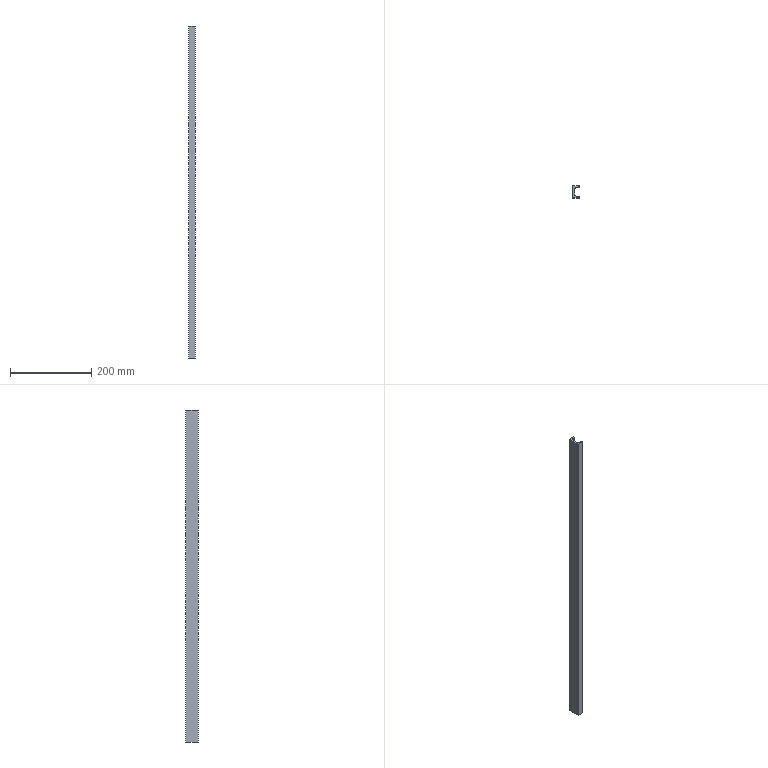Part | STEP file | DIN 1026-1 U 30x15 1785507254409 | 1 solid | 14 faces | box 15 x 30 x 815 mm | volume 180323 mm3 | plane 10 | cylinder 4 | commonest cylinder face diameters 4 x2 9 x2
STEP:
#1=CARTESIAN_POINT('',(4.,-6.066,815.));
#2=VERTEX_POINT('',#1);
#3=CARTESIAN_POINT('',(8.141,-10.551,815.));
#4=VERTEX_POINT('',#3);
#5=CARTESIAN_POINT('',(8.5,-6.066,815.));
#6=DIRECTION('',(0.,0.,1.));
#7=DIRECTION('',(-1.,0.,0.));
#8=AXIS2_PLACEMENT_3D('',#5,#6,#7);
#9=CIRCLE('',#8,4.5);
#10=EDGE_CURVE('',#2,#4,#9,.T.);
#11=ORIENTED_EDGE('',*,*,#10,.T.);
#12=CARTESIAN_POINT('',(8.141,-10.551,0.));
#13=VERTEX_POINT('',#12);
#14=CARTESIAN_POINT('',(8.141,-10.551,0.));
#15=DIRECTION('',(0.,0.,1.));
#16=VECTOR('',#15,10.);
#17=LINE('',#14,#16);
#18=EDGE_CURVE('',#13,#4,#17,.T.);
#19=ORIENTED_EDGE('',*,*,#18,.F.);
#20=CARTESIAN_POINT('',(4.,-6.066,0.));
#21=VERTEX_POINT('',#20);
#22=CARTESIAN_POINT('',(8.5,-6.066,0.));
#23=DIRECTION('',(0.,0.,1.));
#24=DIRECTION('',(-1.,0.,0.));
#25=AXIS2_PLACEMENT_3D('',#22,#23,#24);
#26=CIRCLE('',#25,4.5);
#27=EDGE_CURVE('',#21,#13,#26,.T.);
#28=ORIENTED_EDGE('',*,*,#27,.F.);
#29=CARTESIAN_POINT('',(4.,-6.066,0.));
#30=DIRECTION('',(0.,0.,1.));
#31=VECTOR('',#30,10.);
#32=LINE('',#29,#31);
#33=EDGE_CURVE('',#21,#2,#32,.T.);
#34=ORIENTED_EDGE('',*,*,#33,.T.);
#35=EDGE_LOOP('',(#11,#19,#28,#34));
#36=FACE_OUTER_BOUND('',#35,.T.);
#37=CARTESIAN_POINT('',(8.5,-6.066,0.));
#38=DIRECTION('',(0.,0.,1.));
#39=DIRECTION('',(-1.,0.,0.));
#40=AXIS2_PLACEMENT_3D('',#37,#38,#39);
#41=CYLINDRICAL_SURFACE('',#40,4.5);
#42=ADVANCED_FACE('',(#36),#41,.F.);
#43=CARTESIAN_POINT('',(13.159,-10.953,815.));
#44=VERTEX_POINT('',#43);
#45=CARTESIAN_POINT('',(7.403,-10.492,815.));
#46=DIRECTION('',(0.9968,-0.07975,0.));
#47=VECTOR('',#46,10.);
#48=LINE('',#45,#47);
#49=EDGE_CURVE('',#4,#44,#48,.T.);
#50=ORIENTED_EDGE('',*,*,#49,.T.);
#51=CARTESIAN_POINT('',(13.159,-10.953,0.));
#52=VERTEX_POINT('',#51);
#53=CARTESIAN_POINT('',(13.159,-10.953,0.));
#54=DIRECTION('',(0.,0.,1.));
#55=VECTOR('',#54,10.);
#56=LINE('',#53,#55);
#57=EDGE_CURVE('',#52,#44,#56,.T.);
#58=ORIENTED_EDGE('',*,*,#57,.F.);
#59=CARTESIAN_POINT('',(7.403,-10.492,0.));
#60=DIRECTION('',(0.9968,-0.07975,0.));
#61=VECTOR('',#60,10.);
#62=LINE('',#59,#61);
#63=EDGE_CURVE('',#13,#52,#62,.T.);
#64=ORIENTED_EDGE('',*,*,#63,.F.);
#65=ORIENTED_EDGE('',*,*,#18,.T.);
#66=EDGE_LOOP('',(#50,#58,#64,#65));
#67=FACE_OUTER_BOUND('',#66,.T.);
#68=CARTESIAN_POINT('',(8.141,-10.551,0.));
#69=DIRECTION('',(0.07975,0.9968,0.));
#70=DIRECTION('',(0.,0.,1.));
#71=AXIS2_PLACEMENT_3D('',#68,#69,#70);
#72=PLANE('',#71);
#73=ADVANCED_FACE('',(#67),#72,.T.);
#74=CARTESIAN_POINT('',(15.,-12.946,815.));
#75=VERTEX_POINT('',#74);
#76=CARTESIAN_POINT('',(13.,-12.946,815.));
#77=DIRECTION('',(0.,0.,-1.));
#78=DIRECTION('',(-1.,0.,0.));
#79=AXIS2_PLACEMENT_3D('',#76,#77,#78);
#80=CIRCLE('',#79,2.);
#81=EDGE_CURVE('',#44,#75,#80,.T.);
#82=ORIENTED_EDGE('',*,*,#81,.T.);
#83=CARTESIAN_POINT('',(15.,-12.946,0.));
#84=VERTEX_POINT('',#83);
#85=CARTESIAN_POINT('',(15.,-12.946,0.));
#86=DIRECTION('',(0.,0.,1.));
#87=VECTOR('',#86,10.);
#88=LINE('',#85,#87);
#89=EDGE_CURVE('',#84,#75,#88,.T.);
#90=ORIENTED_EDGE('',*,*,#89,.F.);
#91=CARTESIAN_POINT('',(13.,-12.946,0.));
#92=DIRECTION('',(0.,0.,-1.));
#93=DIRECTION('',(-1.,0.,0.));
#94=AXIS2_PLACEMENT_3D('',#91,#92,#93);
#95=CIRCLE('',#94,2.);
#96=EDGE_CURVE('',#52,#84,#95,.T.);
#97=ORIENTED_EDGE('',*,*,#96,.F.);
#98=ORIENTED_EDGE('',*,*,#57,.T.);
#99=EDGE_LOOP('',(#82,#90,#97,#98));
#100=FACE_OUTER_BOUND('',#99,.T.);
#101=CARTESIAN_POINT('',(13.,-12.946,0.));
#102=DIRECTION('',(0.,0.,1.));
#103=DIRECTION('',(-1.,0.,0.));
#104=AXIS2_PLACEMENT_3D('',#101,#102,#103);
#105=CYLINDRICAL_SURFACE('',#104,2.);
#106=ADVANCED_FACE('',(#100),#105,.T.);
#107=CARTESIAN_POINT('',(15.,-15.,815.));
#108=VERTEX_POINT('',#107);
#109=CARTESIAN_POINT('',(15.,-6.473,815.));
#110=DIRECTION('',(0.,-1.,0.));
#111=VECTOR('',#110,10.);
#112=LINE('',#109,#111);
#113=EDGE_CURVE('',#75,#108,#112,.T.);
#114=ORIENTED_EDGE('',*,*,#113,.T.);
#115=CARTESIAN_POINT('',(15.,-15.,0.));
#116=VERTEX_POINT('',#115);
#117=CARTESIAN_POINT('',(15.,-15.,0.));
#118=DIRECTION('',(0.,0.,1.));
#119=VECTOR('',#118,10.);
#120=LINE('',#117,#119);
#121=EDGE_CURVE('',#116,#108,#120,.T.);
#122=ORIENTED_EDGE('',*,*,#121,.F.);
#123=CARTESIAN_POINT('',(15.,-6.473,0.));
#124=DIRECTION('',(0.,-1.,0.));
#125=VECTOR('',#124,10.);
#126=LINE('',#123,#125);
#127=EDGE_CURVE('',#84,#116,#126,.T.);
#128=ORIENTED_EDGE('',*,*,#127,.F.);
#129=ORIENTED_EDGE('',*,*,#89,.T.);
#130=EDGE_LOOP('',(#114,#122,#128,#129));
#131=FACE_OUTER_BOUND('',#130,.T.);
#132=CARTESIAN_POINT('',(15.,-12.946,0.));
#133=DIRECTION('',(1.,0.,0.));
#134=DIRECTION('',(0.,0.,-1.));
#135=AXIS2_PLACEMENT_3D('',#132,#133,#134);
#136=PLANE('',#135);
#137=ADVANCED_FACE('',(#131),#136,.T.);
#138=CARTESIAN_POINT('',(0.,-15.,815.));
#139=VERTEX_POINT('',#138);
#140=CARTESIAN_POINT('',(11.25,-15.,815.));
#141=DIRECTION('',(-1.,0.,0.));
#142=VECTOR('',#141,10.);
#143=LINE('',#140,#142);
#144=EDGE_CURVE('',#108,#139,#143,.T.);
#145=ORIENTED_EDGE('',*,*,#144,.T.);
#146=CARTESIAN_POINT('',(0.,-15.,0.));
#147=VERTEX_POINT('',#146);
#148=CARTESIAN_POINT('',(0.,-15.,0.));
#149=DIRECTION('',(0.,0.,1.));
#150=VECTOR('',#149,10.);
#151=LINE('',#148,#150);
#152=EDGE_CURVE('',#147,#139,#151,.T.);
#153=ORIENTED_EDGE('',*,*,#152,.F.);
#154=CARTESIAN_POINT('',(11.25,-15.,0.));
#155=DIRECTION('',(-1.,0.,0.));
#156=VECTOR('',#155,10.);
#157=LINE('',#154,#156);
#158=EDGE_CURVE('',#116,#147,#157,.T.);
#159=ORIENTED_EDGE('',*,*,#158,.F.);
#160=ORIENTED_EDGE('',*,*,#121,.T.);
#161=EDGE_LOOP('',(#145,#153,#159,#160));
#162=FACE_OUTER_BOUND('',#161,.T.);
#163=CARTESIAN_POINT('',(15.,-15.,0.));
#164=DIRECTION('',(0.,-1.,0.));
#165=DIRECTION('',(0.,0.,-1.));
#166=AXIS2_PLACEMENT_3D('',#163,#164,#165);
#167=PLANE('',#166);
#168=ADVANCED_FACE('',(#162),#167,.T.);
#169=CARTESIAN_POINT('',(0.,15.,815.));
#170=VERTEX_POINT('',#169);
#171=CARTESIAN_POINT('',(0.,0.,815.));
#172=DIRECTION('',(0.,1.,0.));
#173=VECTOR('',#172,10.);
#174=LINE('',#171,#173);
#175=EDGE_CURVE('',#139,#170,#174,.T.);
#176=ORIENTED_EDGE('',*,*,#175,.T.);
#177=CARTESIAN_POINT('',(0.,15.,0.));
#178=VERTEX_POINT('',#177);
#179=CARTESIAN_POINT('',(0.,15.,0.));
#180=DIRECTION('',(0.,0.,1.));
#181=VECTOR('',#180,10.);
#182=LINE('',#179,#181);
#183=EDGE_CURVE('',#178,#170,#182,.T.);
#184=ORIENTED_EDGE('',*,*,#183,.F.);
#185=CARTESIAN_POINT('',(0.,0.,0.));
#186=DIRECTION('',(0.,1.,0.));
#187=VECTOR('',#186,10.);
#188=LINE('',#185,#187);
#189=EDGE_CURVE('',#147,#178,#188,.T.);
#190=ORIENTED_EDGE('',*,*,#189,.F.);
#191=ORIENTED_EDGE('',*,*,#152,.T.);
#192=EDGE_LOOP('',(#176,#184,#190,#191));
#193=FACE_OUTER_BOUND('',#192,.T.);
#194=CARTESIAN_POINT('',(0.,0.,0.));
#195=DIRECTION('',(-1.,0.,0.));
#196=DIRECTION('',(0.,0.,1.));
#197=AXIS2_PLACEMENT_3D('',#194,#195,#196);
#198=PLANE('',#197);
#199=ADVANCED_FACE('',(#193),#198,.T.);
#200=CARTESIAN_POINT('',(15.,15.,815.));
#201=VERTEX_POINT('',#200);
#202=CARTESIAN_POINT('',(3.75,15.,815.));
#203=DIRECTION('',(1.,0.,0.));
#204=VECTOR('',#203,10.);
#205=LINE('',#202,#204);
#206=EDGE_CURVE('',#170,#201,#205,.T.);
#207=ORIENTED_EDGE('',*,*,#206,.T.);
#208=CARTESIAN_POINT('',(15.,15.,0.));
#209=VERTEX_POINT('',#208);
#210=CARTESIAN_POINT('',(15.,15.,0.));
#211=DIRECTION('',(0.,0.,1.));
#212=VECTOR('',#211,10.);
#213=LINE('',#210,#212);
#214=EDGE_CURVE('',#209,#201,#213,.T.);
#215=ORIENTED_EDGE('',*,*,#214,.F.);
#216=CARTESIAN_POINT('',(3.75,15.,0.));
#217=DIRECTION('',(1.,0.,0.));
#218=VECTOR('',#217,10.);
#219=LINE('',#216,#218);
#220=EDGE_CURVE('',#178,#209,#219,.T.);
#221=ORIENTED_EDGE('',*,*,#220,.F.);
#222=ORIENTED_EDGE('',*,*,#183,.T.);
#223=EDGE_LOOP('',(#207,#215,#221,#222));
#224=FACE_OUTER_BOUND('',#223,.T.);
#225=CARTESIAN_POINT('',(0.,15.,0.));
#226=DIRECTION('',(0.,1.,0.));
#227=DIRECTION('',(0.,0.,1.));
#228=AXIS2_PLACEMENT_3D('',#225,#226,#227);
#229=PLANE('',#228);
#230=ADVANCED_FACE('',(#224),#229,.T.);
#231=CARTESIAN_POINT('',(15.,12.946,815.));
#232=VERTEX_POINT('',#231);
#233=CARTESIAN_POINT('',(15.,7.5,815.));
#234=DIRECTION('',(0.,-1.,0.));
#235=VECTOR('',#234,10.);
#236=LINE('',#233,#235);
#237=EDGE_CURVE('',#201,#232,#236,.T.);
#238=ORIENTED_EDGE('',*,*,#237,.T.);
#239=CARTESIAN_POINT('',(15.,12.946,0.));
#240=VERTEX_POINT('',#239);
#241=CARTESIAN_POINT('',(15.,12.946,0.));
#242=DIRECTION('',(0.,0.,1.));
#243=VECTOR('',#242,10.);
#244=LINE('',#241,#243);
#245=EDGE_CURVE('',#240,#232,#244,.T.);
#246=ORIENTED_EDGE('',*,*,#245,.F.);
#247=CARTESIAN_POINT('',(15.,7.5,0.));
#248=DIRECTION('',(0.,-1.,0.));
#249=VECTOR('',#248,10.);
#250=LINE('',#247,#249);
#251=EDGE_CURVE('',#209,#240,#250,.T.);
#252=ORIENTED_EDGE('',*,*,#251,.F.);
#253=ORIENTED_EDGE('',*,*,#214,.T.);
#254=EDGE_LOOP('',(#238,#246,#252,#253));
#255=FACE_OUTER_BOUND('',#254,.T.);
#256=CARTESIAN_POINT('',(15.,15.,0.));
#257=DIRECTION('',(1.,0.,0.));
#258=DIRECTION('',(0.,0.,-1.));
#259=AXIS2_PLACEMENT_3D('',#256,#257,#258);
#260=PLANE('',#259);
#261=ADVANCED_FACE('',(#255),#260,.T.);
#262=CARTESIAN_POINT('',(13.159,10.953,815.));
#263=VERTEX_POINT('',#262);
#264=CARTESIAN_POINT('',(13.,12.946,815.));
#265=DIRECTION('',(0.,0.,-1.));
#266=DIRECTION('',(-0.07975,0.9968,0.));
#267=AXIS2_PLACEMENT_3D('',#264,#265,#266);
#268=CIRCLE('',#267,2.);
#269=EDGE_CURVE('',#232,#263,#268,.T.);
#270=ORIENTED_EDGE('',*,*,#269,.T.);
#271=CARTESIAN_POINT('',(13.159,10.953,0.));
#272=VERTEX_POINT('',#271);
#273=CARTESIAN_POINT('',(13.159,10.953,0.));
#274=DIRECTION('',(0.,0.,1.));
#275=VECTOR('',#274,10.);
#276=LINE('',#273,#275);
#277=EDGE_CURVE('',#272,#263,#276,.T.);
#278=ORIENTED_EDGE('',*,*,#277,.F.);
#279=CARTESIAN_POINT('',(13.,12.946,0.));
#280=DIRECTION('',(0.,0.,-1.));
#281=DIRECTION('',(-0.07975,0.9968,0.));
#282=AXIS2_PLACEMENT_3D('',#279,#280,#281);
#283=CIRCLE('',#282,2.);
#284=EDGE_CURVE('',#240,#272,#283,.T.);
#285=ORIENTED_EDGE('',*,*,#284,.F.);
#286=ORIENTED_EDGE('',*,*,#245,.T.);
#287=EDGE_LOOP('',(#270,#278,#285,#286));
#288=FACE_OUTER_BOUND('',#287,.T.);
#289=CARTESIAN_POINT('',(13.,12.946,0.));
#290=DIRECTION('',(0.,0.,1.));
#291=DIRECTION('',(-0.07975,0.9968,0.));
#292=AXIS2_PLACEMENT_3D('',#289,#290,#291);
#293=CYLINDRICAL_SURFACE('',#292,2.);
#294=ADVANCED_FACE('',(#288),#293,.T.);
#295=CARTESIAN_POINT('',(8.141,10.551,815.));
#296=VERTEX_POINT('',#295);
#297=CARTESIAN_POINT('',(9.912,10.693,815.));
#298=DIRECTION('',(-0.9968,-0.07975,0.));
#299=VECTOR('',#298,10.);
#300=LINE('',#297,#299);
#301=EDGE_CURVE('',#263,#296,#300,.T.);
#302=ORIENTED_EDGE('',*,*,#301,.T.);
#303=CARTESIAN_POINT('',(8.141,10.551,0.));
#304=VERTEX_POINT('',#303);
#305=CARTESIAN_POINT('',(8.141,10.551,0.));
#306=DIRECTION('',(0.,0.,1.));
#307=VECTOR('',#306,10.);
#308=LINE('',#305,#307);
#309=EDGE_CURVE('',#304,#296,#308,.T.);
#310=ORIENTED_EDGE('',*,*,#309,.F.);
#311=CARTESIAN_POINT('',(9.912,10.693,0.));
#312=DIRECTION('',(-0.9968,-0.07975,0.));
#313=VECTOR('',#312,10.);
#314=LINE('',#311,#313);
#315=EDGE_CURVE('',#272,#304,#314,.T.);
#316=ORIENTED_EDGE('',*,*,#315,.F.);
#317=ORIENTED_EDGE('',*,*,#277,.T.);
#318=EDGE_LOOP('',(#302,#310,#316,#317));
#319=FACE_OUTER_BOUND('',#318,.T.);
#320=CARTESIAN_POINT('',(13.159,10.953,0.));
#321=DIRECTION('',(0.07975,-0.9968,0.));
#322=DIRECTION('',(0.,0.,-1.));
#323=AXIS2_PLACEMENT_3D('',#320,#321,#322);
#324=PLANE('',#323);
#325=ADVANCED_FACE('',(#319),#324,.T.);
#326=CARTESIAN_POINT('',(4.,6.066,815.));
#327=VERTEX_POINT('',#326);
#328=CARTESIAN_POINT('',(8.5,6.066,815.));
#329=DIRECTION('',(0.,0.,1.));
#330=DIRECTION('',(-0.07975,0.9968,0.));
#331=AXIS2_PLACEMENT_3D('',#328,#329,#330);
#332=CIRCLE('',#331,4.5);
#333=EDGE_CURVE('',#296,#327,#332,.T.);
#334=ORIENTED_EDGE('',*,*,#333,.T.);
#335=CARTESIAN_POINT('',(4.,6.066,0.));
#336=VERTEX_POINT('',#335);
#337=CARTESIAN_POINT('',(4.,6.066,0.));
#338=DIRECTION('',(0.,0.,1.));
#339=VECTOR('',#338,10.);
#340=LINE('',#337,#339);
#341=EDGE_CURVE('',#336,#327,#340,.T.);
#342=ORIENTED_EDGE('',*,*,#341,.F.);
#343=CARTESIAN_POINT('',(8.5,6.066,0.));
#344=DIRECTION('',(0.,0.,1.));
#345=DIRECTION('',(-0.07975,0.9968,0.));
#346=AXIS2_PLACEMENT_3D('',#343,#344,#345);
#347=CIRCLE('',#346,4.5);
#348=EDGE_CURVE('',#304,#336,#347,.T.);
#349=ORIENTED_EDGE('',*,*,#348,.F.);
#350=ORIENTED_EDGE('',*,*,#309,.T.);
#351=EDGE_LOOP('',(#334,#342,#349,#350));
#352=FACE_OUTER_BOUND('',#351,.T.);
#353=CARTESIAN_POINT('',(8.5,6.066,0.));
#354=DIRECTION('',(0.,0.,1.));
#355=DIRECTION('',(-0.07975,0.9968,0.));
#356=AXIS2_PLACEMENT_3D('',#353,#354,#355);
#357=CYLINDRICAL_SURFACE('',#356,4.5);
#358=ADVANCED_FACE('',(#352),#357,.F.);
#359=CARTESIAN_POINT('',(4.,0.,815.));
#360=DIRECTION('',(0.,-1.,0.));
#361=VECTOR('',#360,10.);
#362=LINE('',#359,#361);
#363=EDGE_CURVE('',#327,#2,#362,.T.);
#364=ORIENTED_EDGE('',*,*,#363,.T.);
#365=ORIENTED_EDGE('',*,*,#33,.F.);
#366=CARTESIAN_POINT('',(4.,0.,0.));
#367=DIRECTION('',(0.,-1.,0.));
#368=VECTOR('',#367,10.);
#369=LINE('',#366,#368);
#370=EDGE_CURVE('',#336,#21,#369,.T.);
#371=ORIENTED_EDGE('',*,*,#370,.F.);
#372=ORIENTED_EDGE('',*,*,#341,.T.);
#373=EDGE_LOOP('',(#364,#365,#371,#372));
#374=FACE_OUTER_BOUND('',#373,.T.);
#375=CARTESIAN_POINT('',(4.,0.,0.));
#376=DIRECTION('',(1.,0.,0.));
#377=DIRECTION('',(0.,0.,-1.));
#378=AXIS2_PLACEMENT_3D('',#375,#376,#377);
#379=PLANE('',#378);
#380=ADVANCED_FACE('',(#374),#379,.T.);
#381=ORIENTED_EDGE('',*,*,#220,.T.);
#382=ORIENTED_EDGE('',*,*,#251,.T.);
#383=ORIENTED_EDGE('',*,*,#284,.T.);
#384=ORIENTED_EDGE('',*,*,#315,.T.);
#385=ORIENTED_EDGE('',*,*,#348,.T.);
#386=ORIENTED_EDGE('',*,*,#370,.T.);
#387=ORIENTED_EDGE('',*,*,#27,.T.);
#388=ORIENTED_EDGE('',*,*,#63,.T.);
#389=ORIENTED_EDGE('',*,*,#96,.T.);
#390=ORIENTED_EDGE('',*,*,#127,.T.);
#391=ORIENTED_EDGE('',*,*,#158,.T.);
#392=ORIENTED_EDGE('',*,*,#189,.T.);
#393=EDGE_LOOP('',(#381,#382,#383,#384,#385,#386,#387,#388,#389,#390,#391,#392));
#394=FACE_OUTER_BOUND('',#393,.T.);
#395=CARTESIAN_POINT('',(7.5,0.,0.));
#396=DIRECTION('',(0.,0.,1.));
#397=DIRECTION('',(1.,0.,0.));
#398=AXIS2_PLACEMENT_3D('',#395,#396,#397);
#399=PLANE('',#398);
#400=ADVANCED_FACE('',(#394),#399,.F.);
#401=ORIENTED_EDGE('',*,*,#206,.F.);
#402=ORIENTED_EDGE('',*,*,#175,.F.);
#403=ORIENTED_EDGE('',*,*,#144,.F.);
#404=ORIENTED_EDGE('',*,*,#113,.F.);
#405=ORIENTED_EDGE('',*,*,#81,.F.);
#406=ORIENTED_EDGE('',*,*,#49,.F.);
#407=ORIENTED_EDGE('',*,*,#10,.F.);
#408=ORIENTED_EDGE('',*,*,#363,.F.);
#409=ORIENTED_EDGE('',*,*,#333,.F.);
#410=ORIENTED_EDGE('',*,*,#301,.F.);
#411=ORIENTED_EDGE('',*,*,#269,.F.);
#412=ORIENTED_EDGE('',*,*,#237,.F.);
#413=EDGE_LOOP('',(#401,#402,#403,#404,#405,#406,#407,#408,#409,#410,#411,#412));
#414=FACE_OUTER_BOUND('',#413,.T.);
#415=CARTESIAN_POINT('',(7.5,0.,815.));
#416=DIRECTION('',(0.,0.,1.));
#417=DIRECTION('',(1.,0.,0.));
#418=AXIS2_PLACEMENT_3D('',#415,#416,#417);
#419=PLANE('',#418);
#420=ADVANCED_FACE('',(#414),#419,.T.);
#421=CLOSED_SHELL('',(#42,#73,#106,#137,#168,#199,#230,#261,#294,#325,#358,#380,#400,#420));
#422=MANIFOLD_SOLID_BREP('',#421);
#423=(LENGTH_UNIT()NAMED_UNIT(*)SI_UNIT(.MILLI.,.METRE.));
#424=UNCERTAINTY_MEASURE_WITH_UNIT(LENGTH_MEASURE(0.01),#423,'','');
#425=(NAMED_UNIT(*)PLANE_ANGLE_UNIT()SI_UNIT($,.RADIAN.));
#426=(NAMED_UNIT(*)SI_UNIT($,.STERADIAN.)SOLID_ANGLE_UNIT());
#427=(GEOMETRIC_REPRESENTATION_CONTEXT(3)GLOBAL_UNCERTAINTY_ASSIGNED_CONTEXT((#424))GLOBAL_UNIT_ASSIGNED_CONTEXT((#423,#425,#426))REPRESENTATION_CONTEXT('',''));
#428=ADVANCED_BREP_SHAPE_REPRESENTATION('',(#422),#427);